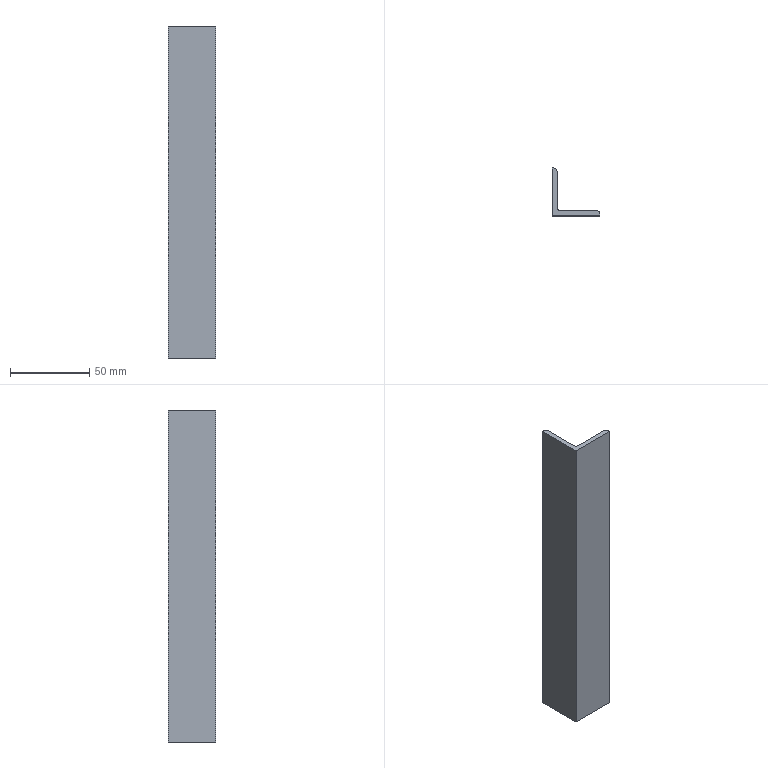Part | SolidWorks | features Extrusion 1 | 1 solid | 11 faces | box 30 x 30 x 210 mm | volume 35730 mm3 | plane 8 | cylinder 3 | commonest cylinder face diameters 4 x3
STEP:
#1=CARTESIAN_POINT('',(0.,30.,0.));
#2=VERTEX_POINT('',#1);
#3=CARTESIAN_POINT('',(0.,0.,0.));
#4=VERTEX_POINT('',#3);
#5=CARTESIAN_POINT('',(0.,0.,0.));
#6=DIRECTION('',(0.,-1.,0.));
#7=VECTOR('',#6,1000.);
#8=LINE('',#5,#7);
#9=EDGE_CURVE('',#2,#4,#8,.T.);
#10=ORIENTED_EDGE('',*,*,#9,.T.);
#11=CARTESIAN_POINT('',(0.,0.,210.));
#12=VERTEX_POINT('',#11);
#13=CARTESIAN_POINT('',(0.,0.,210.));
#14=DIRECTION('',(0.,0.,-1.));
#15=VECTOR('',#14,1000.);
#16=LINE('',#13,#15);
#17=EDGE_CURVE('',#12,#4,#16,.T.);
#18=ORIENTED_EDGE('',*,*,#17,.F.);
#19=CARTESIAN_POINT('',(0.,30.,210.));
#20=VERTEX_POINT('',#19);
#21=CARTESIAN_POINT('',(0.,0.,210.));
#22=DIRECTION('',(0.,-1.,0.));
#23=VECTOR('',#22,1000.);
#24=LINE('',#21,#23);
#25=EDGE_CURVE('',#20,#12,#24,.T.);
#26=ORIENTED_EDGE('',*,*,#25,.F.);
#27=CARTESIAN_POINT('',(0.,30.,210.));
#28=DIRECTION('',(0.,0.,-1.));
#29=VECTOR('',#28,1000.);
#30=LINE('',#27,#29);
#31=EDGE_CURVE('',#20,#2,#30,.T.);
#32=ORIENTED_EDGE('',*,*,#31,.T.);
#33=EDGE_LOOP('',(#10,#18,#26,#32));
#34=FACE_OUTER_BOUND('',#33,.T.);
#35=CARTESIAN_POINT('',(0.,0.,210.));
#36=DIRECTION('',(1.,0.,0.));
#37=DIRECTION('',(0.,0.,-1.));
#38=AXIS2_PLACEMENT_3D('',#35,#36,#37);
#39=PLANE('',#38);
#40=ADVANCED_FACE('',(#34),#39,.F.);
#41=CARTESIAN_POINT('',(30.,0.,0.));
#42=VERTEX_POINT('',#41);
#43=CARTESIAN_POINT('',(0.,0.,0.));
#44=DIRECTION('',(1.,0.,0.));
#45=VECTOR('',#44,1000.);
#46=LINE('',#43,#45);
#47=EDGE_CURVE('',#4,#42,#46,.T.);
#48=ORIENTED_EDGE('',*,*,#47,.T.);
#49=CARTESIAN_POINT('',(30.,0.,210.));
#50=VERTEX_POINT('',#49);
#51=CARTESIAN_POINT('',(30.,0.,210.));
#52=DIRECTION('',(0.,0.,-1.));
#53=VECTOR('',#52,1000.);
#54=LINE('',#51,#53);
#55=EDGE_CURVE('',#50,#42,#54,.T.);
#56=ORIENTED_EDGE('',*,*,#55,.F.);
#57=CARTESIAN_POINT('',(0.,0.,210.));
#58=DIRECTION('',(1.,0.,0.));
#59=VECTOR('',#58,1000.);
#60=LINE('',#57,#59);
#61=EDGE_CURVE('',#12,#50,#60,.T.);
#62=ORIENTED_EDGE('',*,*,#61,.F.);
#63=ORIENTED_EDGE('',*,*,#17,.T.);
#64=EDGE_LOOP('',(#48,#56,#62,#63));
#65=FACE_OUTER_BOUND('',#64,.T.);
#66=CARTESIAN_POINT('',(0.,0.,210.));
#67=DIRECTION('',(0.,1.,0.));
#68=DIRECTION('',(0.,0.,1.));
#69=AXIS2_PLACEMENT_3D('',#66,#67,#68);
#70=PLANE('',#69);
#71=ADVANCED_FACE('',(#65),#70,.F.);
#72=CARTESIAN_POINT('',(30.,1.,0.));
#73=VERTEX_POINT('',#72);
#74=CARTESIAN_POINT('',(30.,1.,0.));
#75=DIRECTION('',(0.,1.,0.));
#76=VECTOR('',#75,1000.);
#77=LINE('',#74,#76);
#78=EDGE_CURVE('',#42,#73,#77,.T.);
#79=ORIENTED_EDGE('',*,*,#78,.T.);
#80=CARTESIAN_POINT('',(30.,1.,210.));
#81=VERTEX_POINT('',#80);
#82=CARTESIAN_POINT('',(30.,1.,210.));
#83=DIRECTION('',(0.,0.,-1.));
#84=VECTOR('',#83,1000.);
#85=LINE('',#82,#84);
#86=EDGE_CURVE('',#81,#73,#85,.T.);
#87=ORIENTED_EDGE('',*,*,#86,.F.);
#88=CARTESIAN_POINT('',(30.,1.,210.));
#89=DIRECTION('',(0.,1.,0.));
#90=VECTOR('',#89,1000.);
#91=LINE('',#88,#90);
#92=EDGE_CURVE('',#50,#81,#91,.T.);
#93=ORIENTED_EDGE('',*,*,#92,.F.);
#94=ORIENTED_EDGE('',*,*,#55,.T.);
#95=EDGE_LOOP('',(#79,#87,#93,#94));
#96=FACE_OUTER_BOUND('',#95,.T.);
#97=CARTESIAN_POINT('',(30.,1.,210.));
#98=DIRECTION('',(-1.,0.,0.));
#99=DIRECTION('',(0.,0.,1.));
#100=AXIS2_PLACEMENT_3D('',#97,#98,#99);
#101=PLANE('',#100);
#102=ADVANCED_FACE('',(#96),#101,.F.);
#103=CARTESIAN_POINT('',(28.,3.,0.));
#104=VERTEX_POINT('',#103);
#105=CARTESIAN_POINT('',(28.,1.,0.));
#106=DIRECTION('',(0.,0.,1.));
#107=DIRECTION('',(1.,0.,0.));
#108=AXIS2_PLACEMENT_3D('',#105,#106,#107);
#109=CIRCLE('',#108,2.);
#110=EDGE_CURVE('',#73,#104,#109,.T.);
#111=ORIENTED_EDGE('',*,*,#110,.T.);
#112=CARTESIAN_POINT('',(28.,3.,210.));
#113=VERTEX_POINT('',#112);
#114=CARTESIAN_POINT('',(28.,3.,210.));
#115=DIRECTION('',(0.,0.,-1.));
#116=VECTOR('',#115,1000.);
#117=LINE('',#114,#116);
#118=EDGE_CURVE('',#113,#104,#117,.T.);
#119=ORIENTED_EDGE('',*,*,#118,.F.);
#120=CARTESIAN_POINT('',(28.,1.,210.));
#121=DIRECTION('',(0.,0.,1.));
#122=DIRECTION('',(1.,0.,0.));
#123=AXIS2_PLACEMENT_3D('',#120,#121,#122);
#124=CIRCLE('',#123,2.);
#125=EDGE_CURVE('',#81,#113,#124,.T.);
#126=ORIENTED_EDGE('',*,*,#125,.F.);
#127=ORIENTED_EDGE('',*,*,#86,.T.);
#128=EDGE_LOOP('',(#111,#119,#126,#127));
#129=FACE_OUTER_BOUND('',#128,.T.);
#130=CARTESIAN_POINT('',(28.,1.,210.));
#131=DIRECTION('',(0.,0.,-1.));
#132=DIRECTION('',(-1.,0.,0.));
#133=AXIS2_PLACEMENT_3D('',#130,#131,#132);
#134=CYLINDRICAL_SURFACE('',#133,2.);
#135=ADVANCED_FACE('',(#129),#134,.T.);
#136=CARTESIAN_POINT('',(5.,3.,0.));
#137=VERTEX_POINT('',#136);
#138=CARTESIAN_POINT('',(5.,3.,0.));
#139=DIRECTION('',(-1.,0.,0.));
#140=VECTOR('',#139,1000.);
#141=LINE('',#138,#140);
#142=EDGE_CURVE('',#104,#137,#141,.T.);
#143=ORIENTED_EDGE('',*,*,#142,.T.);
#144=CARTESIAN_POINT('',(5.,3.,210.));
#145=VERTEX_POINT('',#144);
#146=CARTESIAN_POINT('',(5.,3.,210.));
#147=DIRECTION('',(0.,0.,-1.));
#148=VECTOR('',#147,1000.);
#149=LINE('',#146,#148);
#150=EDGE_CURVE('',#145,#137,#149,.T.);
#151=ORIENTED_EDGE('',*,*,#150,.F.);
#152=CARTESIAN_POINT('',(5.,3.,210.));
#153=DIRECTION('',(-1.,0.,0.));
#154=VECTOR('',#153,1000.);
#155=LINE('',#152,#154);
#156=EDGE_CURVE('',#113,#145,#155,.T.);
#157=ORIENTED_EDGE('',*,*,#156,.F.);
#158=ORIENTED_EDGE('',*,*,#118,.T.);
#159=EDGE_LOOP('',(#143,#151,#157,#158));
#160=FACE_OUTER_BOUND('',#159,.T.);
#161=CARTESIAN_POINT('',(5.,3.,210.));
#162=DIRECTION('',(0.,-1.,0.));
#163=DIRECTION('',(0.,0.,-1.));
#164=AXIS2_PLACEMENT_3D('',#161,#162,#163);
#165=PLANE('',#164);
#166=ADVANCED_FACE('',(#160),#165,.F.);
#167=CARTESIAN_POINT('',(3.,5.,0.));
#168=VERTEX_POINT('',#167);
#169=CARTESIAN_POINT('',(5.,5.,0.));
#170=DIRECTION('',(0.,0.,-1.));
#171=DIRECTION('',(-1.,0.,0.));
#172=AXIS2_PLACEMENT_3D('',#169,#170,#171);
#173=CIRCLE('',#172,2.);
#174=EDGE_CURVE('',#137,#168,#173,.T.);
#175=ORIENTED_EDGE('',*,*,#174,.T.);
#176=CARTESIAN_POINT('',(3.,5.,210.));
#177=VERTEX_POINT('',#176);
#178=CARTESIAN_POINT('',(3.,5.,210.));
#179=DIRECTION('',(0.,0.,-1.));
#180=VECTOR('',#179,1000.);
#181=LINE('',#178,#180);
#182=EDGE_CURVE('',#177,#168,#181,.T.);
#183=ORIENTED_EDGE('',*,*,#182,.F.);
#184=CARTESIAN_POINT('',(5.,5.,210.));
#185=DIRECTION('',(0.,0.,-1.));
#186=DIRECTION('',(-1.,0.,0.));
#187=AXIS2_PLACEMENT_3D('',#184,#185,#186);
#188=CIRCLE('',#187,2.);
#189=EDGE_CURVE('',#145,#177,#188,.T.);
#190=ORIENTED_EDGE('',*,*,#189,.F.);
#191=ORIENTED_EDGE('',*,*,#150,.T.);
#192=EDGE_LOOP('',(#175,#183,#190,#191));
#193=FACE_OUTER_BOUND('',#192,.T.);
#194=CARTESIAN_POINT('',(5.,5.,210.));
#195=DIRECTION('',(0.,0.,-1.));
#196=DIRECTION('',(-1.,0.,0.));
#197=AXIS2_PLACEMENT_3D('',#194,#195,#196);
#198=CYLINDRICAL_SURFACE('',#197,2.);
#199=ADVANCED_FACE('',(#193),#198,.F.);
#200=CARTESIAN_POINT('',(3.,28.,0.));
#201=VERTEX_POINT('',#200);
#202=CARTESIAN_POINT('',(3.,5.,0.));
#203=DIRECTION('',(0.,1.,0.));
#204=VECTOR('',#203,1000.);
#205=LINE('',#202,#204);
#206=EDGE_CURVE('',#168,#201,#205,.T.);
#207=ORIENTED_EDGE('',*,*,#206,.T.);
#208=CARTESIAN_POINT('',(3.,28.,210.));
#209=VERTEX_POINT('',#208);
#210=CARTESIAN_POINT('',(3.,28.,210.));
#211=DIRECTION('',(0.,0.,-1.));
#212=VECTOR('',#211,1000.);
#213=LINE('',#210,#212);
#214=EDGE_CURVE('',#209,#201,#213,.T.);
#215=ORIENTED_EDGE('',*,*,#214,.F.);
#216=CARTESIAN_POINT('',(3.,5.,210.));
#217=DIRECTION('',(0.,1.,0.));
#218=VECTOR('',#217,1000.);
#219=LINE('',#216,#218);
#220=EDGE_CURVE('',#177,#209,#219,.T.);
#221=ORIENTED_EDGE('',*,*,#220,.F.);
#222=ORIENTED_EDGE('',*,*,#182,.T.);
#223=EDGE_LOOP('',(#207,#215,#221,#222));
#224=FACE_OUTER_BOUND('',#223,.T.);
#225=CARTESIAN_POINT('',(3.,5.,210.));
#226=DIRECTION('',(-1.,0.,0.));
#227=DIRECTION('',(0.,0.,1.));
#228=AXIS2_PLACEMENT_3D('',#225,#226,#227);
#229=PLANE('',#228);
#230=ADVANCED_FACE('',(#224),#229,.F.);
#231=CARTESIAN_POINT('',(1.,30.,0.));
#232=VERTEX_POINT('',#231);
#233=CARTESIAN_POINT('',(1.,28.,0.));
#234=DIRECTION('',(0.,0.,1.));
#235=DIRECTION('',(1.,0.,0.));
#236=AXIS2_PLACEMENT_3D('',#233,#234,#235);
#237=CIRCLE('',#236,2.);
#238=EDGE_CURVE('',#201,#232,#237,.T.);
#239=ORIENTED_EDGE('',*,*,#238,.T.);
#240=CARTESIAN_POINT('',(1.,30.,210.));
#241=VERTEX_POINT('',#240);
#242=CARTESIAN_POINT('',(1.,30.,210.));
#243=DIRECTION('',(0.,0.,-1.));
#244=VECTOR('',#243,1000.);
#245=LINE('',#242,#244);
#246=EDGE_CURVE('',#241,#232,#245,.T.);
#247=ORIENTED_EDGE('',*,*,#246,.F.);
#248=CARTESIAN_POINT('',(1.,28.,210.));
#249=DIRECTION('',(0.,0.,1.));
#250=DIRECTION('',(1.,0.,0.));
#251=AXIS2_PLACEMENT_3D('',#248,#249,#250);
#252=CIRCLE('',#251,2.);
#253=EDGE_CURVE('',#209,#241,#252,.T.);
#254=ORIENTED_EDGE('',*,*,#253,.F.);
#255=ORIENTED_EDGE('',*,*,#214,.T.);
#256=EDGE_LOOP('',(#239,#247,#254,#255));
#257=FACE_OUTER_BOUND('',#256,.T.);
#258=CARTESIAN_POINT('',(1.,28.,210.));
#259=DIRECTION('',(0.,0.,-1.));
#260=DIRECTION('',(-1.,0.,0.));
#261=AXIS2_PLACEMENT_3D('',#258,#259,#260);
#262=CYLINDRICAL_SURFACE('',#261,2.);
#263=ADVANCED_FACE('',(#257),#262,.T.);
#264=CARTESIAN_POINT('',(0.,30.,0.));
#265=DIRECTION('',(-1.,0.,0.));
#266=VECTOR('',#265,1000.);
#267=LINE('',#264,#266);
#268=EDGE_CURVE('',#232,#2,#267,.T.);
#269=ORIENTED_EDGE('',*,*,#268,.T.);
#270=ORIENTED_EDGE('',*,*,#31,.F.);
#271=CARTESIAN_POINT('',(0.,30.,210.));
#272=DIRECTION('',(-1.,0.,0.));
#273=VECTOR('',#272,1000.);
#274=LINE('',#271,#273);
#275=EDGE_CURVE('',#241,#20,#274,.T.);
#276=ORIENTED_EDGE('',*,*,#275,.F.);
#277=ORIENTED_EDGE('',*,*,#246,.T.);
#278=EDGE_LOOP('',(#269,#270,#276,#277));
#279=FACE_OUTER_BOUND('',#278,.T.);
#280=CARTESIAN_POINT('',(0.,30.,210.));
#281=DIRECTION('',(0.,-1.,0.));
#282=DIRECTION('',(0.,0.,-1.));
#283=AXIS2_PLACEMENT_3D('',#280,#281,#282);
#284=PLANE('',#283);
#285=ADVANCED_FACE('',(#279),#284,.F.);
#286=ORIENTED_EDGE('',*,*,#25,.T.);
#287=ORIENTED_EDGE('',*,*,#61,.T.);
#288=ORIENTED_EDGE('',*,*,#92,.T.);
#289=ORIENTED_EDGE('',*,*,#125,.T.);
#290=ORIENTED_EDGE('',*,*,#156,.T.);
#291=ORIENTED_EDGE('',*,*,#189,.T.);
#292=ORIENTED_EDGE('',*,*,#220,.T.);
#293=ORIENTED_EDGE('',*,*,#253,.T.);
#294=ORIENTED_EDGE('',*,*,#275,.T.);
#295=EDGE_LOOP('',(#286,#287,#288,#289,#290,#291,#292,#293,#294));
#296=FACE_OUTER_BOUND('',#295,.T.);
#297=CARTESIAN_POINT('',(1.,28.,210.));
#298=DIRECTION('',(0.,0.,1.));
#299=DIRECTION('',(1.,0.,0.));
#300=AXIS2_PLACEMENT_3D('',#297,#298,#299);
#301=PLANE('',#300);
#302=ADVANCED_FACE('',(#296),#301,.T.);
#303=ORIENTED_EDGE('',*,*,#9,.F.);
#304=ORIENTED_EDGE('',*,*,#268,.F.);
#305=ORIENTED_EDGE('',*,*,#238,.F.);
#306=ORIENTED_EDGE('',*,*,#206,.F.);
#307=ORIENTED_EDGE('',*,*,#174,.F.);
#308=ORIENTED_EDGE('',*,*,#142,.F.);
#309=ORIENTED_EDGE('',*,*,#110,.F.);
#310=ORIENTED_EDGE('',*,*,#78,.F.);
#311=ORIENTED_EDGE('',*,*,#47,.F.);
#312=EDGE_LOOP('',(#303,#304,#305,#306,#307,#308,#309,#310,#311));
#313=FACE_OUTER_BOUND('',#312,.T.);
#314=CARTESIAN_POINT('',(1.,28.,0.));
#315=DIRECTION('',(0.,0.,1.));
#316=DIRECTION('',(1.,0.,0.));
#317=AXIS2_PLACEMENT_3D('',#314,#315,#316);
#318=PLANE('',#317);
#319=ADVANCED_FACE('',(#313),#318,.F.);
#320=CLOSED_SHELL('',(#40,#71,#102,#135,#166,#199,#230,#263,#285,#302,#319));
#321=MANIFOLD_SOLID_BREP('',#320);
#322=CARTESIAN_POINT('',(0.,0.,0.));
#323=DIRECTION('',(0.,0.,1.));
#324=DIRECTION('',(1.,0.,0.));
#325=AXIS2_PLACEMENT_3D('',#322,#323,#324);
#326=(LENGTH_UNIT()NAMED_UNIT(*)SI_UNIT(.MILLI.,.METRE.));
#327=UNCERTAINTY_MEASURE_WITH_UNIT(LENGTH_MEASURE(0.00001),#326,'','');
#328=(NAMED_UNIT(*)PLANE_ANGLE_UNIT()SI_UNIT($,.RADIAN.));
#329=(NAMED_UNIT(*)SI_UNIT($,.STERADIAN.)SOLID_ANGLE_UNIT());
#330=(GEOMETRIC_REPRESENTATION_CONTEXT(3)GLOBAL_UNCERTAINTY_ASSIGNED_CONTEXT((#327))GLOBAL_UNIT_ASSIGNED_CONTEXT((#326,#328,#329))REPRESENTATION_CONTEXT('',''));
#331=ADVANCED_BREP_SHAPE_REPRESENTATION('',(#321,#325),#330);